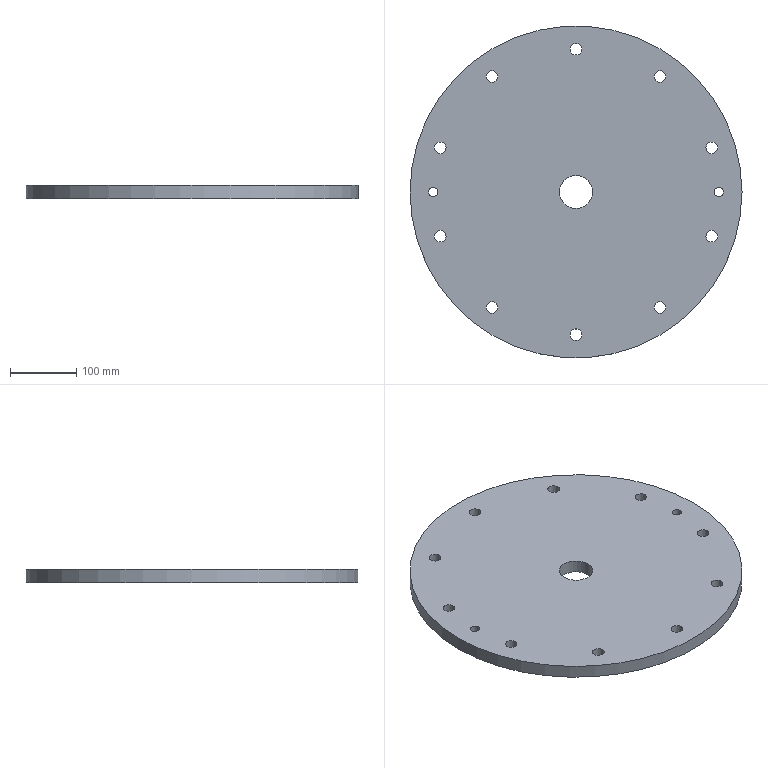Part | NX | 1 solid | 16 faces | box 500 x 500 x 20 mm | volume 3833458 mm3 | cylinder 14 | plane 2 | commonest cylinder face diameters 17.5 x10 14 x2 50 x1 500 x1
STEP:
#1=CARTESIAN_POINT('',(-207.181,-58.117,-20.));
#2=VERTEX_POINT('',#1);
#3=CARTESIAN_POINT('',(-204.477,-66.439,-20.));
#4=DIRECTION('',(0.,0.,1.));
#5=DIRECTION('',(-0.309,0.9511,0.));
#6=AXIS2_PLACEMENT_3D('',#3,#4,#5);
#7=CIRCLE('',#6,8.75);
#8=EDGE_CURVE('',#2,#2,#7,.T.);
#9=ORIENTED_EDGE('',*,*,#8,.F.);
#10=EDGE_LOOP('',(#9));
#11=FACE_BOUND('',#10,.T.);
#12=CARTESIAN_POINT('',(-207.181,-58.117,0.));
#13=VERTEX_POINT('',#12);
#14=CARTESIAN_POINT('',(-204.477,-66.439,0.));
#15=DIRECTION('',(0.,0.,1.));
#16=DIRECTION('',(-0.309,0.9511,0.));
#17=AXIS2_PLACEMENT_3D('',#14,#15,#16);
#18=CIRCLE('',#17,8.75);
#19=EDGE_CURVE('',#13,#13,#18,.T.);
#20=ORIENTED_EDGE('',*,*,#19,.T.);
#21=EDGE_LOOP('',(#20));
#22=FACE_BOUND('',#21,.T.);
#23=CARTESIAN_POINT('',(-204.477,-66.439,-20.));
#24=DIRECTION('',(0.,0.,1.));
#25=DIRECTION('',(1.,0.,0.));
#26=AXIS2_PLACEMENT_3D('',#23,#24,#25);
#27=CYLINDRICAL_SURFACE('',#26,8.75);
#28=ADVANCED_FACE('',(#11,#22),#27,.F.);
#29=CARTESIAN_POINT('',(-201.773,74.76,-20.));
#30=VERTEX_POINT('',#29);
#31=CARTESIAN_POINT('',(-204.477,66.439,-20.));
#32=DIRECTION('',(0.,0.,1.));
#33=DIRECTION('',(0.309,0.9511,0.));
#34=AXIS2_PLACEMENT_3D('',#31,#32,#33);
#35=CIRCLE('',#34,8.75);
#36=EDGE_CURVE('',#30,#30,#35,.T.);
#37=ORIENTED_EDGE('',*,*,#36,.F.);
#38=EDGE_LOOP('',(#37));
#39=FACE_BOUND('',#38,.T.);
#40=CARTESIAN_POINT('',(-201.773,74.76,0.));
#41=VERTEX_POINT('',#40);
#42=CARTESIAN_POINT('',(-204.477,66.439,0.));
#43=DIRECTION('',(0.,0.,1.));
#44=DIRECTION('',(0.309,0.9511,0.));
#45=AXIS2_PLACEMENT_3D('',#42,#43,#44);
#46=CIRCLE('',#45,8.75);
#47=EDGE_CURVE('',#41,#41,#46,.T.);
#48=ORIENTED_EDGE('',*,*,#47,.T.);
#49=EDGE_LOOP('',(#48));
#50=FACE_BOUND('',#49,.T.);
#51=CARTESIAN_POINT('',(-204.477,66.439,-20.));
#52=DIRECTION('',(0.,0.,1.));
#53=DIRECTION('',(1.,0.,0.));
#54=AXIS2_PLACEMENT_3D('',#51,#52,#53);
#55=CYLINDRICAL_SURFACE('',#54,8.75);
#56=ADVANCED_FACE('',(#39,#50),#55,.F.);
#57=CARTESIAN_POINT('',(-133.453,-168.796,-20.));
#58=VERTEX_POINT('',#57);
#59=CARTESIAN_POINT('',(-126.374,-173.939,-20.));
#60=DIRECTION('',(0.,0.,1.));
#61=DIRECTION('',(-0.809,0.5878,0.));
#62=AXIS2_PLACEMENT_3D('',#59,#60,#61);
#63=CIRCLE('',#62,8.75);
#64=EDGE_CURVE('',#58,#58,#63,.T.);
#65=ORIENTED_EDGE('',*,*,#64,.F.);
#66=EDGE_LOOP('',(#65));
#67=FACE_BOUND('',#66,.T.);
#68=CARTESIAN_POINT('',(-133.453,-168.796,0.));
#69=VERTEX_POINT('',#68);
#70=CARTESIAN_POINT('',(-126.374,-173.939,0.));
#71=DIRECTION('',(0.,0.,1.));
#72=DIRECTION('',(-0.809,0.5878,0.));
#73=AXIS2_PLACEMENT_3D('',#70,#71,#72);
#74=CIRCLE('',#73,8.75);
#75=EDGE_CURVE('',#69,#69,#74,.T.);
#76=ORIENTED_EDGE('',*,*,#75,.T.);
#77=EDGE_LOOP('',(#76));
#78=FACE_BOUND('',#77,.T.);
#79=CARTESIAN_POINT('',(-126.374,-173.939,-20.));
#80=DIRECTION('',(0.,0.,1.));
#81=DIRECTION('',(1.,0.,0.));
#82=AXIS2_PLACEMENT_3D('',#79,#80,#81);
#83=CYLINDRICAL_SURFACE('',#82,8.75);
#84=ADVANCED_FACE('',(#67,#78),#83,.F.);
#85=CARTESIAN_POINT('',(-119.295,179.082,-20.));
#86=VERTEX_POINT('',#85);
#87=CARTESIAN_POINT('',(-126.374,173.939,-20.));
#88=DIRECTION('',(0.,0.,1.));
#89=DIRECTION('',(0.809,0.5878,0.));
#90=AXIS2_PLACEMENT_3D('',#87,#88,#89);
#91=CIRCLE('',#90,8.75);
#92=EDGE_CURVE('',#86,#86,#91,.T.);
#93=ORIENTED_EDGE('',*,*,#92,.F.);
#94=EDGE_LOOP('',(#93));
#95=FACE_BOUND('',#94,.T.);
#96=CARTESIAN_POINT('',(-119.295,179.082,0.));
#97=VERTEX_POINT('',#96);
#98=CARTESIAN_POINT('',(-126.374,173.939,0.));
#99=DIRECTION('',(0.,0.,1.));
#100=DIRECTION('',(0.809,0.5878,0.));
#101=AXIS2_PLACEMENT_3D('',#98,#99,#100);
#102=CIRCLE('',#101,8.75);
#103=EDGE_CURVE('',#97,#97,#102,.T.);
#104=ORIENTED_EDGE('',*,*,#103,.T.);
#105=EDGE_LOOP('',(#104));
#106=FACE_BOUND('',#105,.T.);
#107=CARTESIAN_POINT('',(-126.374,173.939,-20.));
#108=DIRECTION('',(0.,0.,1.));
#109=DIRECTION('',(1.,0.,0.));
#110=AXIS2_PLACEMENT_3D('',#107,#108,#109);
#111=CYLINDRICAL_SURFACE('',#110,8.75);
#112=ADVANCED_FACE('',(#95,#106),#111,.F.);
#113=CARTESIAN_POINT('',(25.,0.,-20.));
#114=VERTEX_POINT('',#113);
#115=CARTESIAN_POINT('',(0.,0.,-20.));
#116=DIRECTION('',(0.,0.,1.));
#117=DIRECTION('',(1.,0.,0.));
#118=AXIS2_PLACEMENT_3D('',#115,#116,#117);
#119=CIRCLE('',#118,25.);
#120=EDGE_CURVE('',#114,#114,#119,.T.);
#121=ORIENTED_EDGE('',*,*,#120,.F.);
#122=EDGE_LOOP('',(#121));
#123=FACE_BOUND('',#122,.T.);
#124=CARTESIAN_POINT('',(25.,0.,0.));
#125=VERTEX_POINT('',#124);
#126=CARTESIAN_POINT('',(0.,0.,0.));
#127=DIRECTION('',(0.,0.,1.));
#128=DIRECTION('',(1.,0.,0.));
#129=AXIS2_PLACEMENT_3D('',#126,#127,#128);
#130=CIRCLE('',#129,25.);
#131=EDGE_CURVE('',#125,#125,#130,.T.);
#132=ORIENTED_EDGE('',*,*,#131,.T.);
#133=EDGE_LOOP('',(#132));
#134=FACE_BOUND('',#133,.T.);
#135=CARTESIAN_POINT('',(0.,0.,-20.));
#136=DIRECTION('',(0.,0.,1.));
#137=DIRECTION('',(1.,0.,0.));
#138=AXIS2_PLACEMENT_3D('',#135,#136,#137);
#139=CYLINDRICAL_SURFACE('',#138,25.);
#140=ADVANCED_FACE('',(#123,#134),#139,.F.);
#141=CARTESIAN_POINT('',(-8.75,-215.,-20.));
#142=VERTEX_POINT('',#141);
#143=CARTESIAN_POINT('',(0.,-215.,-20.));
#144=DIRECTION('',(0.,0.,1.));
#145=DIRECTION('',(-1.,0.,0.));
#146=AXIS2_PLACEMENT_3D('',#143,#144,#145);
#147=CIRCLE('',#146,8.75);
#148=EDGE_CURVE('',#142,#142,#147,.T.);
#149=ORIENTED_EDGE('',*,*,#148,.F.);
#150=EDGE_LOOP('',(#149));
#151=FACE_BOUND('',#150,.T.);
#152=CARTESIAN_POINT('',(-8.75,-215.,0.));
#153=VERTEX_POINT('',#152);
#154=CARTESIAN_POINT('',(0.,-215.,0.));
#155=DIRECTION('',(0.,0.,1.));
#156=DIRECTION('',(-1.,0.,0.));
#157=AXIS2_PLACEMENT_3D('',#154,#155,#156);
#158=CIRCLE('',#157,8.75);
#159=EDGE_CURVE('',#153,#153,#158,.T.);
#160=ORIENTED_EDGE('',*,*,#159,.T.);
#161=EDGE_LOOP('',(#160));
#162=FACE_BOUND('',#161,.T.);
#163=CARTESIAN_POINT('',(0.,-215.,-20.));
#164=DIRECTION('',(0.,0.,1.));
#165=DIRECTION('',(1.,0.,0.));
#166=AXIS2_PLACEMENT_3D('',#163,#164,#165);
#167=CYLINDRICAL_SURFACE('',#166,8.75);
#168=ADVANCED_FACE('',(#151,#162),#167,.F.);
#169=CARTESIAN_POINT('',(8.75,215.,-20.));
#170=VERTEX_POINT('',#169);
#171=CARTESIAN_POINT('',(0.,215.,-20.));
#172=DIRECTION('',(0.,0.,1.));
#173=DIRECTION('',(1.,0.,0.));
#174=AXIS2_PLACEMENT_3D('',#171,#172,#173);
#175=CIRCLE('',#174,8.75);
#176=EDGE_CURVE('',#170,#170,#175,.T.);
#177=ORIENTED_EDGE('',*,*,#176,.F.);
#178=EDGE_LOOP('',(#177));
#179=FACE_BOUND('',#178,.T.);
#180=CARTESIAN_POINT('',(8.75,215.,0.));
#181=VERTEX_POINT('',#180);
#182=CARTESIAN_POINT('',(0.,215.,0.));
#183=DIRECTION('',(0.,0.,1.));
#184=DIRECTION('',(1.,0.,0.));
#185=AXIS2_PLACEMENT_3D('',#182,#183,#184);
#186=CIRCLE('',#185,8.75);
#187=EDGE_CURVE('',#181,#181,#186,.T.);
#188=ORIENTED_EDGE('',*,*,#187,.T.);
#189=EDGE_LOOP('',(#188));
#190=FACE_BOUND('',#189,.T.);
#191=CARTESIAN_POINT('',(0.,215.,-20.));
#192=DIRECTION('',(0.,0.,1.));
#193=DIRECTION('',(1.,0.,0.));
#194=AXIS2_PLACEMENT_3D('',#191,#192,#193);
#195=CYLINDRICAL_SURFACE('',#194,8.75);
#196=ADVANCED_FACE('',(#179,#190),#195,.F.);
#197=CARTESIAN_POINT('',(119.295,-179.082,-20.));
#198=VERTEX_POINT('',#197);
#199=CARTESIAN_POINT('',(126.374,-173.939,-20.));
#200=DIRECTION('',(0.,0.,1.));
#201=DIRECTION('',(-0.809,-0.5878,0.));
#202=AXIS2_PLACEMENT_3D('',#199,#200,#201);
#203=CIRCLE('',#202,8.75);
#204=EDGE_CURVE('',#198,#198,#203,.T.);
#205=ORIENTED_EDGE('',*,*,#204,.F.);
#206=EDGE_LOOP('',(#205));
#207=FACE_BOUND('',#206,.T.);
#208=CARTESIAN_POINT('',(119.295,-179.082,0.));
#209=VERTEX_POINT('',#208);
#210=CARTESIAN_POINT('',(126.374,-173.939,0.));
#211=DIRECTION('',(0.,0.,1.));
#212=DIRECTION('',(-0.809,-0.5878,0.));
#213=AXIS2_PLACEMENT_3D('',#210,#211,#212);
#214=CIRCLE('',#213,8.75);
#215=EDGE_CURVE('',#209,#209,#214,.T.);
#216=ORIENTED_EDGE('',*,*,#215,.T.);
#217=EDGE_LOOP('',(#216));
#218=FACE_BOUND('',#217,.T.);
#219=CARTESIAN_POINT('',(126.374,-173.939,-20.));
#220=DIRECTION('',(0.,0.,1.));
#221=DIRECTION('',(1.,0.,0.));
#222=AXIS2_PLACEMENT_3D('',#219,#220,#221);
#223=CYLINDRICAL_SURFACE('',#222,8.75);
#224=ADVANCED_FACE('',(#207,#218),#223,.F.);
#225=CARTESIAN_POINT('',(133.453,168.796,-20.));
#226=VERTEX_POINT('',#225);
#227=CARTESIAN_POINT('',(126.374,173.939,-20.));
#228=DIRECTION('',(0.,0.,1.));
#229=DIRECTION('',(0.809,-0.5878,0.));
#230=AXIS2_PLACEMENT_3D('',#227,#228,#229);
#231=CIRCLE('',#230,8.75);
#232=EDGE_CURVE('',#226,#226,#231,.T.);
#233=ORIENTED_EDGE('',*,*,#232,.F.);
#234=EDGE_LOOP('',(#233));
#235=FACE_BOUND('',#234,.T.);
#236=CARTESIAN_POINT('',(133.453,168.796,0.));
#237=VERTEX_POINT('',#236);
#238=CARTESIAN_POINT('',(126.374,173.939,0.));
#239=DIRECTION('',(0.,0.,1.));
#240=DIRECTION('',(0.809,-0.5878,0.));
#241=AXIS2_PLACEMENT_3D('',#238,#239,#240);
#242=CIRCLE('',#241,8.75);
#243=EDGE_CURVE('',#237,#237,#242,.T.);
#244=ORIENTED_EDGE('',*,*,#243,.T.);
#245=EDGE_LOOP('',(#244));
#246=FACE_BOUND('',#245,.T.);
#247=CARTESIAN_POINT('',(126.374,173.939,-20.));
#248=DIRECTION('',(0.,0.,1.));
#249=DIRECTION('',(1.,0.,0.));
#250=AXIS2_PLACEMENT_3D('',#247,#248,#249);
#251=CYLINDRICAL_SURFACE('',#250,8.75);
#252=ADVANCED_FACE('',(#235,#246),#251,.F.);
#253=CARTESIAN_POINT('',(201.773,-74.76,-20.));
#254=VERTEX_POINT('',#253);
#255=CARTESIAN_POINT('',(204.477,-66.439,-20.));
#256=DIRECTION('',(0.,0.,1.));
#257=DIRECTION('',(-0.309,-0.9511,0.));
#258=AXIS2_PLACEMENT_3D('',#255,#256,#257);
#259=CIRCLE('',#258,8.75);
#260=EDGE_CURVE('',#254,#254,#259,.T.);
#261=ORIENTED_EDGE('',*,*,#260,.F.);
#262=EDGE_LOOP('',(#261));
#263=FACE_BOUND('',#262,.T.);
#264=CARTESIAN_POINT('',(201.773,-74.76,0.));
#265=VERTEX_POINT('',#264);
#266=CARTESIAN_POINT('',(204.477,-66.439,0.));
#267=DIRECTION('',(0.,0.,1.));
#268=DIRECTION('',(-0.309,-0.9511,0.));
#269=AXIS2_PLACEMENT_3D('',#266,#267,#268);
#270=CIRCLE('',#269,8.75);
#271=EDGE_CURVE('',#265,#265,#270,.T.);
#272=ORIENTED_EDGE('',*,*,#271,.T.);
#273=EDGE_LOOP('',(#272));
#274=FACE_BOUND('',#273,.T.);
#275=CARTESIAN_POINT('',(204.477,-66.439,-20.));
#276=DIRECTION('',(0.,0.,1.));
#277=DIRECTION('',(1.,0.,0.));
#278=AXIS2_PLACEMENT_3D('',#275,#276,#277);
#279=CYLINDRICAL_SURFACE('',#278,8.75);
#280=ADVANCED_FACE('',(#263,#274),#279,.F.);
#281=CARTESIAN_POINT('',(207.181,58.117,-20.));
#282=VERTEX_POINT('',#281);
#283=CARTESIAN_POINT('',(204.477,66.439,-20.));
#284=DIRECTION('',(0.,0.,1.));
#285=DIRECTION('',(0.309,-0.9511,0.));
#286=AXIS2_PLACEMENT_3D('',#283,#284,#285);
#287=CIRCLE('',#286,8.75);
#288=EDGE_CURVE('',#282,#282,#287,.T.);
#289=ORIENTED_EDGE('',*,*,#288,.F.);
#290=EDGE_LOOP('',(#289));
#291=FACE_BOUND('',#290,.T.);
#292=CARTESIAN_POINT('',(207.181,58.117,0.));
#293=VERTEX_POINT('',#292);
#294=CARTESIAN_POINT('',(204.477,66.439,0.));
#295=DIRECTION('',(0.,0.,1.));
#296=DIRECTION('',(0.309,-0.9511,0.));
#297=AXIS2_PLACEMENT_3D('',#294,#295,#296);
#298=CIRCLE('',#297,8.75);
#299=EDGE_CURVE('',#293,#293,#298,.T.);
#300=ORIENTED_EDGE('',*,*,#299,.T.);
#301=EDGE_LOOP('',(#300));
#302=FACE_BOUND('',#301,.T.);
#303=CARTESIAN_POINT('',(204.477,66.439,-20.));
#304=DIRECTION('',(0.,0.,1.));
#305=DIRECTION('',(1.,0.,0.));
#306=AXIS2_PLACEMENT_3D('',#303,#304,#305);
#307=CYLINDRICAL_SURFACE('',#306,8.75);
#308=ADVANCED_FACE('',(#291,#302),#307,.F.);
#309=CARTESIAN_POINT('',(222.,0.,-20.));
#310=VERTEX_POINT('',#309);
#311=CARTESIAN_POINT('',(215.,0.,-20.));
#312=DIRECTION('',(0.,0.,1.));
#313=DIRECTION('',(1.,0.,0.));
#314=AXIS2_PLACEMENT_3D('',#311,#312,#313);
#315=CIRCLE('',#314,7.);
#316=EDGE_CURVE('',#310,#310,#315,.T.);
#317=ORIENTED_EDGE('',*,*,#316,.F.);
#318=EDGE_LOOP('',(#317));
#319=FACE_BOUND('',#318,.T.);
#320=CARTESIAN_POINT('',(222.,0.,0.));
#321=VERTEX_POINT('',#320);
#322=CARTESIAN_POINT('',(215.,0.,0.));
#323=DIRECTION('',(0.,0.,1.));
#324=DIRECTION('',(1.,0.,0.));
#325=AXIS2_PLACEMENT_3D('',#322,#323,#324);
#326=CIRCLE('',#325,7.);
#327=EDGE_CURVE('',#321,#321,#326,.T.);
#328=ORIENTED_EDGE('',*,*,#327,.T.);
#329=EDGE_LOOP('',(#328));
#330=FACE_BOUND('',#329,.T.);
#331=CARTESIAN_POINT('',(215.,0.,-20.));
#332=DIRECTION('',(0.,0.,1.));
#333=DIRECTION('',(1.,0.,0.));
#334=AXIS2_PLACEMENT_3D('',#331,#332,#333);
#335=CYLINDRICAL_SURFACE('',#334,7.);
#336=ADVANCED_FACE('',(#319,#330),#335,.F.);
#337=CARTESIAN_POINT('',(250.,0.,-20.));
#338=VERTEX_POINT('',#337);
#339=CARTESIAN_POINT('',(0.,0.,-20.));
#340=DIRECTION('',(0.,0.,1.));
#341=DIRECTION('',(1.,0.,0.));
#342=AXIS2_PLACEMENT_3D('',#339,#340,#341);
#343=CIRCLE('',#342,250.);
#344=EDGE_CURVE('',#338,#338,#343,.T.);
#345=ORIENTED_EDGE('',*,*,#344,.T.);
#346=EDGE_LOOP('',(#345));
#347=FACE_BOUND('',#346,.T.);
#348=CARTESIAN_POINT('',(250.,0.,0.));
#349=VERTEX_POINT('',#348);
#350=CARTESIAN_POINT('',(0.,0.,0.));
#351=DIRECTION('',(0.,0.,1.));
#352=DIRECTION('',(1.,0.,0.));
#353=AXIS2_PLACEMENT_3D('',#350,#351,#352);
#354=CIRCLE('',#353,250.);
#355=EDGE_CURVE('',#349,#349,#354,.T.);
#356=ORIENTED_EDGE('',*,*,#355,.F.);
#357=EDGE_LOOP('',(#356));
#358=FACE_BOUND('',#357,.T.);
#359=CARTESIAN_POINT('',(0.,0.,-20.));
#360=DIRECTION('',(0.,0.,1.));
#361=DIRECTION('',(1.,0.,0.));
#362=AXIS2_PLACEMENT_3D('',#359,#360,#361);
#363=CYLINDRICAL_SURFACE('',#362,250.);
#364=ADVANCED_FACE('',(#347,#358),#363,.T.);
#365=CARTESIAN_POINT('',(-208.,0.,-20.));
#366=VERTEX_POINT('',#365);
#367=CARTESIAN_POINT('',(-215.,0.,-20.));
#368=DIRECTION('',(0.,0.,1.));
#369=DIRECTION('',(1.,0.,0.));
#370=AXIS2_PLACEMENT_3D('',#367,#368,#369);
#371=CIRCLE('',#370,7.);
#372=EDGE_CURVE('',#366,#366,#371,.T.);
#373=ORIENTED_EDGE('',*,*,#372,.F.);
#374=EDGE_LOOP('',(#373));
#375=FACE_BOUND('',#374,.T.);
#376=CARTESIAN_POINT('',(-208.,0.,0.));
#377=VERTEX_POINT('',#376);
#378=CARTESIAN_POINT('',(-215.,0.,0.));
#379=DIRECTION('',(0.,0.,1.));
#380=DIRECTION('',(1.,0.,0.));
#381=AXIS2_PLACEMENT_3D('',#378,#379,#380);
#382=CIRCLE('',#381,7.);
#383=EDGE_CURVE('',#377,#377,#382,.T.);
#384=ORIENTED_EDGE('',*,*,#383,.T.);
#385=EDGE_LOOP('',(#384));
#386=FACE_BOUND('',#385,.T.);
#387=CARTESIAN_POINT('',(-215.,0.,-20.));
#388=DIRECTION('',(0.,0.,1.));
#389=DIRECTION('',(1.,0.,0.));
#390=AXIS2_PLACEMENT_3D('',#387,#388,#389);
#391=CYLINDRICAL_SURFACE('',#390,7.);
#392=ADVANCED_FACE('',(#375,#386),#391,.F.);
#393=ORIENTED_EDGE('',*,*,#344,.F.);
#394=EDGE_LOOP('',(#393));
#395=FACE_BOUND('',#394,.T.);
#396=ORIENTED_EDGE('',*,*,#316,.T.);
#397=EDGE_LOOP('',(#396));
#398=FACE_BOUND('',#397,.T.);
#399=ORIENTED_EDGE('',*,*,#288,.T.);
#400=EDGE_LOOP('',(#399));
#401=FACE_BOUND('',#400,.T.);
#402=ORIENTED_EDGE('',*,*,#260,.T.);
#403=EDGE_LOOP('',(#402));
#404=FACE_BOUND('',#403,.T.);
#405=ORIENTED_EDGE('',*,*,#232,.T.);
#406=EDGE_LOOP('',(#405));
#407=FACE_BOUND('',#406,.T.);
#408=ORIENTED_EDGE('',*,*,#204,.T.);
#409=EDGE_LOOP('',(#408));
#410=FACE_BOUND('',#409,.T.);
#411=ORIENTED_EDGE('',*,*,#176,.T.);
#412=EDGE_LOOP('',(#411));
#413=FACE_BOUND('',#412,.T.);
#414=ORIENTED_EDGE('',*,*,#148,.T.);
#415=EDGE_LOOP('',(#414));
#416=FACE_BOUND('',#415,.T.);
#417=ORIENTED_EDGE('',*,*,#120,.T.);
#418=EDGE_LOOP('',(#417));
#419=FACE_BOUND('',#418,.T.);
#420=ORIENTED_EDGE('',*,*,#92,.T.);
#421=EDGE_LOOP('',(#420));
#422=FACE_BOUND('',#421,.T.);
#423=ORIENTED_EDGE('',*,*,#64,.T.);
#424=EDGE_LOOP('',(#423));
#425=FACE_BOUND('',#424,.T.);
#426=ORIENTED_EDGE('',*,*,#36,.T.);
#427=EDGE_LOOP('',(#426));
#428=FACE_BOUND('',#427,.T.);
#429=ORIENTED_EDGE('',*,*,#8,.T.);
#430=EDGE_LOOP('',(#429));
#431=FACE_BOUND('',#430,.T.);
#432=ORIENTED_EDGE('',*,*,#372,.T.);
#433=EDGE_LOOP('',(#432));
#434=FACE_BOUND('',#433,.T.);
#435=CARTESIAN_POINT('',(107.5,0.,-20.));
#436=DIRECTION('',(0.,0.,1.));
#437=DIRECTION('',(1.,0.,0.));
#438=AXIS2_PLACEMENT_3D('',#435,#436,#437);
#439=PLANE('',#438);
#440=ADVANCED_FACE('',(#395,#398,#401,#404,#407,#410,#413,#416,#419,#422,#425,#428,#431,#434),#439,.F.);
#441=ORIENTED_EDGE('',*,*,#355,.T.);
#442=EDGE_LOOP('',(#441));
#443=FACE_BOUND('',#442,.T.);
#444=ORIENTED_EDGE('',*,*,#327,.F.);
#445=EDGE_LOOP('',(#444));
#446=FACE_BOUND('',#445,.T.);
#447=ORIENTED_EDGE('',*,*,#299,.F.);
#448=EDGE_LOOP('',(#447));
#449=FACE_BOUND('',#448,.T.);
#450=ORIENTED_EDGE('',*,*,#271,.F.);
#451=EDGE_LOOP('',(#450));
#452=FACE_BOUND('',#451,.T.);
#453=ORIENTED_EDGE('',*,*,#243,.F.);
#454=EDGE_LOOP('',(#453));
#455=FACE_BOUND('',#454,.T.);
#456=ORIENTED_EDGE('',*,*,#215,.F.);
#457=EDGE_LOOP('',(#456));
#458=FACE_BOUND('',#457,.T.);
#459=ORIENTED_EDGE('',*,*,#187,.F.);
#460=EDGE_LOOP('',(#459));
#461=FACE_BOUND('',#460,.T.);
#462=ORIENTED_EDGE('',*,*,#159,.F.);
#463=EDGE_LOOP('',(#462));
#464=FACE_BOUND('',#463,.T.);
#465=ORIENTED_EDGE('',*,*,#131,.F.);
#466=EDGE_LOOP('',(#465));
#467=FACE_BOUND('',#466,.T.);
#468=ORIENTED_EDGE('',*,*,#103,.F.);
#469=EDGE_LOOP('',(#468));
#470=FACE_BOUND('',#469,.T.);
#471=ORIENTED_EDGE('',*,*,#75,.F.);
#472=EDGE_LOOP('',(#471));
#473=FACE_BOUND('',#472,.T.);
#474=ORIENTED_EDGE('',*,*,#47,.F.);
#475=EDGE_LOOP('',(#474));
#476=FACE_BOUND('',#475,.T.);
#477=ORIENTED_EDGE('',*,*,#19,.F.);
#478=EDGE_LOOP('',(#477));
#479=FACE_BOUND('',#478,.T.);
#480=ORIENTED_EDGE('',*,*,#383,.F.);
#481=EDGE_LOOP('',(#480));
#482=FACE_BOUND('',#481,.T.);
#483=CARTESIAN_POINT('',(107.5,0.,0.));
#484=DIRECTION('',(0.,0.,1.));
#485=DIRECTION('',(1.,0.,0.));
#486=AXIS2_PLACEMENT_3D('',#483,#484,#485);
#487=PLANE('',#486);
#488=ADVANCED_FACE('',(#443,#446,#449,#452,#455,#458,#461,#464,#467,#470,#473,#476,#479,#482),#487,.T.);
#489=CLOSED_SHELL('',(#28,#56,#84,#112,#140,#168,#196,#224,#252,#280,#308,#336,#364,#392,#440,#488));
#490=MANIFOLD_SOLID_BREP('',#489);
#491=(LENGTH_UNIT()NAMED_UNIT(*)SI_UNIT(.MILLI.,.METRE.));
#492=UNCERTAINTY_MEASURE_WITH_UNIT(LENGTH_MEASURE(0.00001),#491,'','');
#493=(NAMED_UNIT(*)PLANE_ANGLE_UNIT()SI_UNIT($,.RADIAN.));
#494=(NAMED_UNIT(*)SI_UNIT($,.STERADIAN.)SOLID_ANGLE_UNIT());
#495=(GEOMETRIC_REPRESENTATION_CONTEXT(3)GLOBAL_UNCERTAINTY_ASSIGNED_CONTEXT((#492))GLOBAL_UNIT_ASSIGNED_CONTEXT((#491,#493,#494))REPRESENTATION_CONTEXT('',''));
#496=ADVANCED_BREP_SHAPE_REPRESENTATION('',(#490),#495);